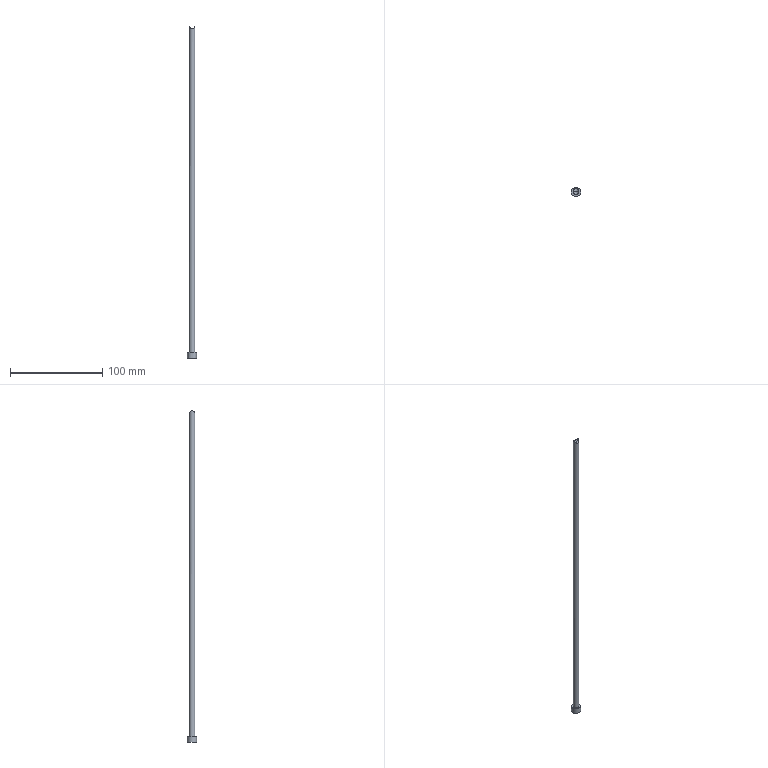Part | NX | features solid 2 | 1 solid | 7 faces | box 10 x 10 x 360.85 mm | volume 10434 mm3 | cylinder 4 | plane 3 | commonest cylinder face diameters 6 x3 10 x1
STEP:
#1=CARTESIAN_POINT('',(3.,0.,-339.5));
#2=VERTEX_POINT('',#1);
#3=CARTESIAN_POINT('',(0.,0.,-339.5));
#4=DIRECTION('',(0.,0.,1.));
#5=DIRECTION('',(1.,0.,0.));
#6=AXIS2_PLACEMENT_3D('',#3,#4,#5);
#7=CIRCLE('',#6,3.);
#8=EDGE_CURVE('',#2,#2,#7,.T.);
#9=ORIENTED_EDGE('',*,*,#8,.T.);
#10=EDGE_LOOP('',(#9));
#11=FACE_BOUND('',#10,.T.);
#12=CARTESIAN_POINT('',(-3.,0.,15.328));
#13=VERTEX_POINT('',#12);
#14=CARTESIAN_POINT('',(3.,0.04487,15.35));
#15=VERTEX_POINT('',#14);
#16=CARTESIAN_POINT('',(-3.,0.,15.328));
#17=CARTESIAN_POINT('',(-3.,0.05591,15.35));
#18=CARTESIAN_POINT('',(-2.997,0.1531,15.24));
#19=CARTESIAN_POINT('',(-2.985,0.3201,15.092));
#20=CARTESIAN_POINT('',(-2.956,0.532,14.879));
#21=CARTESIAN_POINT('',(-2.9,0.7812,14.637));
#22=CARTESIAN_POINT('',(-2.796,1.11,14.313));
#23=CARTESIAN_POINT('',(-2.614,1.504,13.924));
#24=CARTESIAN_POINT('',(-2.192,2.106,13.33));
#25=CARTESIAN_POINT('',(-1.412,2.756,12.686));
#26=CARTESIAN_POINT('',(-0.0151,3.12,12.319));
#27=CARTESIAN_POINT('',(1.395,2.766,12.656));
#28=CARTESIAN_POINT('',(2.341,1.988,13.422));
#29=CARTESIAN_POINT('',(2.787,1.191,14.18));
#30=CARTESIAN_POINT('',(2.966,0.5547,14.852));
#31=CARTESIAN_POINT('',(2.998,0.1638,15.144));
#32=CARTESIAN_POINT('',(3.,0.04487,15.35));
#33=B_SPLINE_CURVE_WITH_KNOTS('',3,(#16,#17,#18,#19,#20,#21,#22,#23,#24,#25,#26,#27,#28,#29,#30,#31,#32),.UNSPECIFIED.,.F.,.F.,(4,1,1,1,1,1,1,1,1,1,1,1,1,1,4),(0.0001498,0.0003287,0.0005076,0.0008655,0.001223,0.001581,0.002297,0.003013,0.004444,0.005876,0.007307,0.008739,0.01017,0.01089,0.0116),.UNSPECIFIED.);
#34=EDGE_CURVE('',#13,#15,#33,.T.);
#35=ORIENTED_EDGE('',*,*,#34,.T.);
#36=CARTESIAN_POINT('',(3.,-0.04487,15.35));
#37=VERTEX_POINT('',#36);
#38=CARTESIAN_POINT('',(0.,0.,15.35));
#39=DIRECTION('',(0.,0.,1.));
#40=DIRECTION('',(1.,0.,0.));
#41=AXIS2_PLACEMENT_3D('',#38,#39,#40);
#42=CIRCLE('',#41,3.);
#43=EDGE_CURVE('',#15,#37,#42,.F.);
#44=ORIENTED_EDGE('',*,*,#43,.T.);
#45=CARTESIAN_POINT('',(3.,-0.04487,15.35));
#46=CARTESIAN_POINT('',(2.998,-0.1631,15.146));
#47=CARTESIAN_POINT('',(2.966,-0.5541,14.853));
#48=CARTESIAN_POINT('',(2.787,-1.189,14.182));
#49=CARTESIAN_POINT('',(2.344,-1.985,13.425));
#50=CARTESIAN_POINT('',(1.4,-2.763,12.659));
#51=CARTESIAN_POINT('',(-0.008458,-3.12,12.319));
#52=CARTESIAN_POINT('',(-1.409,-2.758,12.684));
#53=CARTESIAN_POINT('',(-2.189,-2.108,13.328));
#54=CARTESIAN_POINT('',(-2.61,-1.512,13.917));
#55=CARTESIAN_POINT('',(-2.796,-1.111,14.312));
#56=CARTESIAN_POINT('',(-2.9,-0.7825,14.635));
#57=CARTESIAN_POINT('',(-2.956,-0.5325,14.879));
#58=CARTESIAN_POINT('',(-2.985,-0.3199,15.092));
#59=CARTESIAN_POINT('',(-2.997,-0.1529,15.24));
#60=CARTESIAN_POINT('',(-3.,-0.05555,15.349));
#61=CARTESIAN_POINT('',(-3.,0.,15.328));
#62=B_SPLINE_CURVE_WITH_KNOTS('',3,(#45,#46,#47,#48,#49,#50,#51,#52,#53,#54,#55,#56,#57,#58,#59,#60,#61),.UNSPECIFIED.,.F.,.F.,(4,1,1,1,1,1,1,1,1,1,1,1,1,1,4),(0.01182,0.01254,0.01326,0.0147,0.01614,0.01758,0.01902,0.02046,0.02118,0.0219,0.02226,0.02262,0.02298,0.02316,0.02334),.UNSPECIFIED.);
#63=EDGE_CURVE('',#37,#13,#62,.T.);
#64=ORIENTED_EDGE('',*,*,#63,.T.);
#65=EDGE_LOOP('',(#35,#44,#64));
#66=FACE_BOUND('',#65,.T.);
#67=CARTESIAN_POINT('',(0.,0.,-345.5));
#68=DIRECTION('',(0.,0.,1.));
#69=DIRECTION('',(1.,0.,0.));
#70=AXIS2_PLACEMENT_3D('',#67,#68,#69);
#71=CYLINDRICAL_SURFACE('',#70,3.);
#72=ADVANCED_FACE('',(#11,#66),#71,.T.);
#73=CARTESIAN_POINT('',(2.999,0.,15.35));
#74=VERTEX_POINT('',#73);
#75=CARTESIAN_POINT('',(-0.0004823,0.,15.387));
#76=DIRECTION('',(0.,1.,0.));
#77=DIRECTION('',(-0.3808,0.,-0.9247));
#78=AXIS2_PLACEMENT_3D('',#75,#76,#77);
#79=ELLIPSE('',#78,3.,3.);
#80=EDGE_CURVE('',#13,#74,#79,.F.);
#81=ORIENTED_EDGE('',*,*,#80,.T.);
#82=CARTESIAN_POINT('',(-0.01552,-2.172,15.35));
#83=DIRECTION('',(0.,0.,1.));
#84=DIRECTION('',(-0.006923,-1.,0.));
#85=AXIS2_PLACEMENT_3D('',#82,#83,#84);
#86=ELLIPSE('',#85,178.484,3.);
#87=EDGE_CURVE('',#15,#74,#86,.F.);
#88=ORIENTED_EDGE('',*,*,#87,.F.);
#89=ORIENTED_EDGE('',*,*,#34,.F.);
#90=EDGE_LOOP('',(#81,#88,#89));
#91=FACE_BOUND('',#90,.T.);
#92=CARTESIAN_POINT('',(0.004771,0.7587,15.399));
#93=DIRECTION('',(-0.006922,-0.9998,-0.01681));
#94=DIRECTION('',(0.,-0.01681,0.9999));
#95=AXIS2_PLACEMENT_3D('',#92,#93,#94);
#96=CYLINDRICAL_SURFACE('',#95,3.);
#97=ADVANCED_FACE('',(#91),#96,.F.);
#98=ORIENTED_EDGE('',*,*,#63,.F.);
#99=CARTESIAN_POINT('',(-0.01552,2.172,15.35));
#100=DIRECTION('',(0.,0.,1.));
#101=DIRECTION('',(-0.006923,1.,0.));
#102=AXIS2_PLACEMENT_3D('',#99,#100,#101);
#103=ELLIPSE('',#102,178.484,3.);
#104=EDGE_CURVE('',#37,#74,#103,.T.);
#105=ORIENTED_EDGE('',*,*,#104,.T.);
#106=ORIENTED_EDGE('',*,*,#80,.F.);
#107=EDGE_LOOP('',(#98,#105,#106));
#108=FACE_BOUND('',#107,.T.);
#109=CARTESIAN_POINT('',(0.004771,-0.7587,15.399));
#110=DIRECTION('',(-0.006922,0.9998,-0.01681));
#111=DIRECTION('',(0.,0.01681,0.9999));
#112=AXIS2_PLACEMENT_3D('',#109,#110,#111);
#113=CYLINDRICAL_SURFACE('',#112,3.);
#114=ADVANCED_FACE('',(#108),#113,.F.);
#115=ORIENTED_EDGE('',*,*,#8,.F.);
#116=EDGE_LOOP('',(#115));
#117=FACE_BOUND('',#116,.T.);
#118=CARTESIAN_POINT('',(5.,0.,-339.5));
#119=VERTEX_POINT('',#118);
#120=CARTESIAN_POINT('',(0.,0.,-339.5));
#121=DIRECTION('',(0.,0.,-1.));
#122=DIRECTION('',(1.,0.,0.));
#123=AXIS2_PLACEMENT_3D('',#120,#121,#122);
#124=CIRCLE('',#123,5.);
#125=EDGE_CURVE('',#119,#119,#124,.T.);
#126=ORIENTED_EDGE('',*,*,#125,.F.);
#127=EDGE_LOOP('',(#126));
#128=FACE_BOUND('',#127,.T.);
#129=CARTESIAN_POINT('',(0.,0.,-339.5));
#130=DIRECTION('',(0.,0.,1.));
#131=DIRECTION('',(1.,0.,0.));
#132=AXIS2_PLACEMENT_3D('',#129,#130,#131);
#133=PLANE('',#132);
#134=ADVANCED_FACE('',(#117,#128),#133,.T.);
#135=CARTESIAN_POINT('',(5.,0.,-345.5));
#136=VERTEX_POINT('',#135);
#137=CARTESIAN_POINT('',(0.,0.,-345.5));
#138=DIRECTION('',(0.,0.,1.));
#139=DIRECTION('',(1.,0.,0.));
#140=AXIS2_PLACEMENT_3D('',#137,#138,#139);
#141=CIRCLE('',#140,5.);
#142=EDGE_CURVE('',#136,#136,#141,.T.);
#143=ORIENTED_EDGE('',*,*,#142,.F.);
#144=EDGE_LOOP('',(#143));
#145=FACE_BOUND('',#144,.T.);
#146=CARTESIAN_POINT('',(0.,0.,-345.5));
#147=DIRECTION('',(0.,0.,-1.));
#148=DIRECTION('',(-1.,0.,0.));
#149=AXIS2_PLACEMENT_3D('',#146,#147,#148);
#150=PLANE('',#149);
#151=ADVANCED_FACE('',(#145),#150,.T.);
#152=ORIENTED_EDGE('',*,*,#125,.T.);
#153=EDGE_LOOP('',(#152));
#154=FACE_BOUND('',#153,.T.);
#155=ORIENTED_EDGE('',*,*,#142,.T.);
#156=EDGE_LOOP('',(#155));
#157=FACE_BOUND('',#156,.T.);
#158=CARTESIAN_POINT('',(0.,0.,-345.5));
#159=DIRECTION('',(0.,0.,1.));
#160=DIRECTION('',(1.,0.,0.));
#161=AXIS2_PLACEMENT_3D('',#158,#159,#160);
#162=CYLINDRICAL_SURFACE('',#161,5.);
#163=ADVANCED_FACE('',(#154,#157),#162,.T.);
#164=ORIENTED_EDGE('',*,*,#43,.F.);
#165=ORIENTED_EDGE('',*,*,#87,.T.);
#166=ORIENTED_EDGE('',*,*,#104,.F.);
#167=EDGE_LOOP('',(#164,#165,#166));
#168=FACE_BOUND('',#167,.T.);
#169=CARTESIAN_POINT('',(0.,0.,15.35));
#170=DIRECTION('',(0.,0.,1.));
#171=DIRECTION('',(1.,0.,0.));
#172=AXIS2_PLACEMENT_3D('',#169,#170,#171);
#173=PLANE('',#172);
#174=ADVANCED_FACE('',(#168),#173,.T.);
#175=CLOSED_SHELL('',(#72,#97,#114,#134,#151,#163,#174));
#176=MANIFOLD_SOLID_BREP('',#175);
#177=(LENGTH_UNIT()NAMED_UNIT(*)SI_UNIT(.MILLI.,.METRE.));
#178=UNCERTAINTY_MEASURE_WITH_UNIT(LENGTH_MEASURE(0.0508),#177,'','');
#179=(NAMED_UNIT(*)PLANE_ANGLE_UNIT()SI_UNIT($,.RADIAN.));
#180=(NAMED_UNIT(*)SI_UNIT($,.STERADIAN.)SOLID_ANGLE_UNIT());
#181=(GEOMETRIC_REPRESENTATION_CONTEXT(3)GLOBAL_UNCERTAINTY_ASSIGNED_CONTEXT((#178))GLOBAL_UNIT_ASSIGNED_CONTEXT((#177,#179,#180))REPRESENTATION_CONTEXT('',''));
#182=ADVANCED_BREP_SHAPE_REPRESENTATION('',(#176),#181);